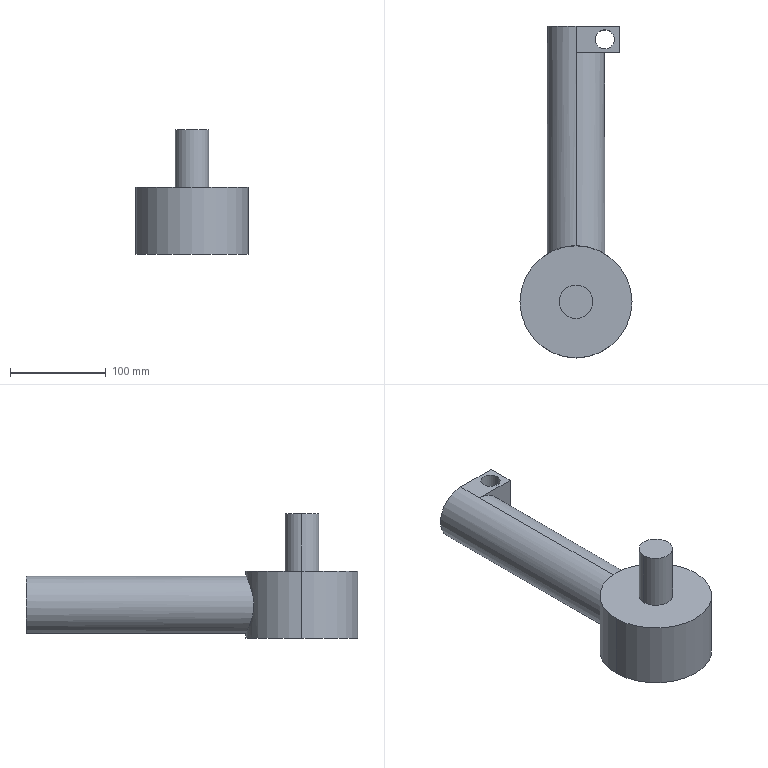Part | SolidWorks | features ICE 4, Extrusion 1 | 1 solid | 16 faces | box 117 x 346.5 x 130 mm | volume 1482010 mm3 | cylinder 8 | plane 8 | commonest cylinder face diameters 20 x2 35 x2 60 x2 117 x2
STEP:
#1=CARTESIAN_POINT('',(40.,274.,65.));
#2=VERTEX_POINT('',#1);
#3=CARTESIAN_POINT('',(20.,274.,65.));
#4=VERTEX_POINT('',#3);
#5=CARTESIAN_POINT('',(30.,274.,65.));
#6=DIRECTION('',(0.,0.,-1.));
#7=DIRECTION('',(-1.,0.,0.));
#8=AXIS2_PLACEMENT_3D('',#5,#6,#7);
#9=CIRCLE('',#8,10.);
#10=EDGE_CURVE('',#2,#4,#9,.T.);
#11=ORIENTED_EDGE('',*,*,#10,.F.);
#12=CARTESIAN_POINT('',(40.,274.,5.));
#13=VERTEX_POINT('',#12);
#14=CARTESIAN_POINT('',(40.,274.,130.));
#15=DIRECTION('',(0.,0.,-1.));
#16=VECTOR('',#15,1000.);
#17=LINE('',#14,#16);
#18=EDGE_CURVE('',#2,#13,#17,.T.);
#19=ORIENTED_EDGE('',*,*,#18,.T.);
#20=CARTESIAN_POINT('',(20.,274.,5.));
#21=VERTEX_POINT('',#20);
#22=CARTESIAN_POINT('',(30.,274.,5.));
#23=DIRECTION('',(0.,0.,-1.));
#24=DIRECTION('',(-1.,0.,0.));
#25=AXIS2_PLACEMENT_3D('',#22,#23,#24);
#26=CIRCLE('',#25,10.);
#27=EDGE_CURVE('',#13,#21,#26,.T.);
#28=ORIENTED_EDGE('',*,*,#27,.T.);
#29=CARTESIAN_POINT('',(20.,274.,130.));
#30=DIRECTION('',(0.,0.,-1.));
#31=VECTOR('',#30,1000.);
#32=LINE('',#29,#31);
#33=EDGE_CURVE('',#4,#21,#32,.T.);
#34=ORIENTED_EDGE('',*,*,#33,.F.);
#35=EDGE_LOOP('',(#11,#19,#28,#34));
#36=FACE_OUTER_BOUND('',#35,.T.);
#37=CARTESIAN_POINT('',(30.,274.,130.));
#38=DIRECTION('',(0.,0.,-1.));
#39=DIRECTION('',(-1.,0.,0.));
#40=AXIS2_PLACEMENT_3D('',#37,#38,#39);
#41=CYLINDRICAL_SURFACE('',#40,10.);
#42=ADVANCED_FACE('',(#36),#41,.F.);
#43=CARTESIAN_POINT('',(17.5,0.,130.));
#44=VERTEX_POINT('',#43);
#45=CARTESIAN_POINT('',(-17.5,0.,130.));
#46=VERTEX_POINT('',#45);
#47=CARTESIAN_POINT('',(0.,0.,130.));
#48=DIRECTION('',(0.,0.,1.));
#49=DIRECTION('',(1.,0.,0.));
#50=AXIS2_PLACEMENT_3D('',#47,#48,#49);
#51=CIRCLE('',#50,17.5);
#52=EDGE_CURVE('',#44,#46,#51,.T.);
#53=ORIENTED_EDGE('',*,*,#52,.F.);
#54=CARTESIAN_POINT('',(17.5,0.,70.));
#55=VERTEX_POINT('',#54);
#56=CARTESIAN_POINT('',(17.5,0.,130.));
#57=DIRECTION('',(0.,0.,-1.));
#58=VECTOR('',#57,1000.);
#59=LINE('',#56,#58);
#60=EDGE_CURVE('',#44,#55,#59,.T.);
#61=ORIENTED_EDGE('',*,*,#60,.T.);
#62=CARTESIAN_POINT('',(-17.5,0.,70.));
#63=VERTEX_POINT('',#62);
#64=CARTESIAN_POINT('',(0.,0.,70.));
#65=DIRECTION('',(0.,0.,1.));
#66=DIRECTION('',(1.,0.,0.));
#67=AXIS2_PLACEMENT_3D('',#64,#65,#66);
#68=CIRCLE('',#67,17.5);
#69=EDGE_CURVE('',#55,#63,#68,.T.);
#70=ORIENTED_EDGE('',*,*,#69,.T.);
#71=CARTESIAN_POINT('',(-17.5,0.,130.));
#72=DIRECTION('',(0.,0.,-1.));
#73=VECTOR('',#72,1000.);
#74=LINE('',#71,#73);
#75=EDGE_CURVE('',#46,#63,#74,.T.);
#76=ORIENTED_EDGE('',*,*,#75,.F.);
#77=EDGE_LOOP('',(#53,#61,#70,#76));
#78=FACE_OUTER_BOUND('',#77,.T.);
#79=CARTESIAN_POINT('',(0.,0.,130.));
#80=DIRECTION('',(0.,0.,-1.));
#81=DIRECTION('',(-1.,0.,0.));
#82=AXIS2_PLACEMENT_3D('',#79,#80,#81);
#83=CYLINDRICAL_SURFACE('',#82,17.5);
#84=ADVANCED_FACE('',(#78),#83,.T.);
#85=CARTESIAN_POINT('',(0.,260.,65.));
#86=VERTEX_POINT('',#85);
#87=CARTESIAN_POINT('',(0.,260.,5.));
#88=VERTEX_POINT('',#87);
#89=CARTESIAN_POINT('',(0.,260.,35.));
#90=DIRECTION('',(0.,1.,0.));
#91=DIRECTION('',(0.,0.,1.));
#92=AXIS2_PLACEMENT_3D('',#89,#90,#91);
#93=CIRCLE('',#92,30.);
#94=EDGE_CURVE('',#86,#88,#93,.T.);
#95=ORIENTED_EDGE('',*,*,#94,.F.);
#96=CARTESIAN_POINT('',(0.,58.5,65.));
#97=VERTEX_POINT('',#96);
#98=CARTESIAN_POINT('',(0.,260.,65.));
#99=DIRECTION('',(0.,-1.,0.));
#100=VECTOR('',#99,1000.);
#101=LINE('',#98,#100);
#102=EDGE_CURVE('',#86,#97,#101,.T.);
#103=ORIENTED_EDGE('',*,*,#102,.T.);
#104=CARTESIAN_POINT('',(0.,58.5,5.));
#105=VERTEX_POINT('',#104);
#106=CARTESIAN_POINT('',(0.,58.5,65.));
#107=CARTESIAN_POINT('',(0.9956,58.5,65.));
#108=CARTESIAN_POINT('',(1.997,58.475,64.95));
#109=CARTESIAN_POINT('',(4.002,58.372,64.749));
#110=CARTESIAN_POINT('',(4.989,58.295,64.599));
#111=CARTESIAN_POINT('',(7.906,57.996,64.007));
#112=CARTESIAN_POINT('',(9.794,57.704,63.425));
#113=CARTESIAN_POINT('',(13.45,56.963,61.889));
#114=CARTESIAN_POINT('',(15.161,56.526,60.959));
#115=CARTESIAN_POINT('',(17.571,55.805,59.335));
#116=CARTESIAN_POINT('',(18.348,55.554,58.755));
#117=CARTESIAN_POINT('',(19.849,55.036,57.516));
#118=CARTESIAN_POINT('',(20.565,54.771,56.863));
#119=CARTESIAN_POINT('',(22.603,53.977,54.819));
#120=CARTESIAN_POINT('',(23.822,53.443,53.337));
#121=CARTESIAN_POINT('',(25.443,52.681,50.925));
#122=CARTESIAN_POINT('',(25.95,52.432,50.084));
#123=CARTESIAN_POINT('',(26.873,51.965,48.371));
#124=CARTESIAN_POINT('',(27.291,51.746,47.495));
#125=CARTESIAN_POINT('',(28.418,51.141,44.807));
#126=CARTESIAN_POINT('',(29.,50.808,42.936));
#127=CARTESIAN_POINT('',(29.499,50.518,40.484));
#128=CARTESIAN_POINT('',(29.587,50.467,39.989));
#129=CARTESIAN_POINT('',(29.736,50.379,39.001));
#130=CARTESIAN_POINT('',(29.799,50.342,38.506));
#131=CARTESIAN_POINT('',(29.948,50.253,37.021));
#132=CARTESIAN_POINT('',(29.999,50.223,36.03));
#133=CARTESIAN_POINT('',(30.001,50.221,34.044));
#134=CARTESIAN_POINT('',(29.953,50.25,33.049));
#135=CARTESIAN_POINT('',(29.806,50.338,31.555));
#136=CARTESIAN_POINT('',(29.744,50.374,31.055));
#137=CARTESIAN_POINT('',(29.595,50.462,30.061));
#138=CARTESIAN_POINT('',(29.508,50.512,29.569));
#139=CARTESIAN_POINT('',(29.018,50.798,27.13));
#140=CARTESIAN_POINT('',(28.439,51.129,25.249));
#141=CARTESIAN_POINT('',(27.491,51.639,22.979));
#142=CARTESIAN_POINT('',(27.289,51.746,22.528));
#143=CARTESIAN_POINT('',(26.866,51.967,21.641));
#144=CARTESIAN_POINT('',(26.645,52.08,21.205));
#145=CARTESIAN_POINT('',(25.952,52.431,19.919));
#146=CARTESIAN_POINT('',(25.452,52.676,19.09));
#147=CARTESIAN_POINT('',(24.376,53.183,17.487));
#148=CARTESIAN_POINT('',(23.801,53.444,16.712));
#149=CARTESIAN_POINT('',(22.572,53.974,15.215));
#150=CARTESIAN_POINT('',(21.917,54.244,14.492));
#151=CARTESIAN_POINT('',(19.871,55.041,12.442));
#152=CARTESIAN_POINT('',(18.39,55.56,11.218));
#153=CARTESIAN_POINT('',(15.981,56.281,9.592));
#154=CARTESIAN_POINT('',(15.146,56.512,9.085));
#155=CARTESIAN_POINT('',(13.414,56.948,8.148));
#156=CARTESIAN_POINT('',(12.529,57.15,7.724));
#157=CARTESIAN_POINT('',(9.824,57.699,6.586));
#158=CARTESIAN_POINT('',(7.948,57.991,6.004));
#159=CARTESIAN_POINT('',(5.02,58.292,5.406));
#160=CARTESIAN_POINT('',(4.02,58.37,5.254));
#161=CARTESIAN_POINT('',(2.518,58.448,5.102));
#162=CARTESIAN_POINT('',(2.016,58.467,5.064));
#163=CARTESIAN_POINT('',(1.01,58.493,5.013));
#164=CARTESIAN_POINT('',(0.5043,58.5,5.));
#165=CARTESIAN_POINT('',(0.,58.5,5.));
#166=B_SPLINE_CURVE_WITH_KNOTS('',3,(#106,#107,#108,#109,#110,#111,#112,#113,#114,#115,#116,#117,#118,#119,#120,#121,#122,#123,#124,#125,#126,#127,#128,#129,#130,#131,#132,#133,#134,#135,#136,#137,#138,#139,#140,#141,#142,#143,#144,#145,#146,#147,#148,#149,#150,#151,#152,#153,#154,#155,#156,#157,#158,#159,#160,#161,#162,#163,#164,#165),.UNSPECIFIED.,.F.,.F.,(4,2,2,2,2,2,2,2,2,2,2,2,2,2,2,2,2,2,2,2,2,2,2,2,2,2,2,2,2,4),(0.09553,0.0985,0.1015,0.1074,0.1134,0.1164,0.1194,0.1253,0.1283,0.1313,0.1372,0.1387,0.1402,0.1432,0.1462,0.1477,0.1492,0.1551,0.1566,0.1581,0.1611,0.1641,0.167,0.173,0.176,0.179,0.1849,0.1879,0.1894,0.1909),.UNSPECIFIED.);
#167=EDGE_CURVE('',#97,#105,#166,.T.);
#168=ORIENTED_EDGE('',*,*,#167,.T.);
#169=CARTESIAN_POINT('',(0.,260.,5.));
#170=DIRECTION('',(0.,-1.,0.));
#171=VECTOR('',#170,1000.);
#172=LINE('',#169,#171);
#173=EDGE_CURVE('',#88,#105,#172,.T.);
#174=ORIENTED_EDGE('',*,*,#173,.F.);
#175=EDGE_LOOP('',(#95,#103,#168,#174));
#176=FACE_OUTER_BOUND('',#175,.T.);
#177=CARTESIAN_POINT('',(0.,260.,35.));
#178=DIRECTION('',(0.,-1.,0.));
#179=DIRECTION('',(0.,0.,-1.));
#180=AXIS2_PLACEMENT_3D('',#177,#178,#179);
#181=CYLINDRICAL_SURFACE('',#180,30.);
#182=ADVANCED_FACE('',(#176),#181,.T.);
#183=CARTESIAN_POINT('',(0.,58.5,5.));
#184=CARTESIAN_POINT('',(-2.021,58.5,5.));
#185=CARTESIAN_POINT('',(-4.002,58.396,5.202));
#186=CARTESIAN_POINT('',(-6.917,58.098,5.791));
#187=CARTESIAN_POINT('',(-7.879,57.975,6.036));
#188=CARTESIAN_POINT('',(-9.307,57.757,6.476));
#189=CARTESIAN_POINT('',(-9.781,57.678,6.635));
#190=CARTESIAN_POINT('',(-10.712,57.513,6.973));
#191=CARTESIAN_POINT('',(-11.171,57.425,7.153));
#192=CARTESIAN_POINT('',(-13.436,56.966,8.105));
#193=CARTESIAN_POINT('',(-15.147,56.53,9.031));
#194=CARTESIAN_POINT('',(-17.17,55.925,10.394));
#195=CARTESIAN_POINT('',(-17.569,55.801,10.678));
#196=CARTESIAN_POINT('',(-18.349,55.549,11.261));
#197=CARTESIAN_POINT('',(-18.731,55.422,11.561));
#198=CARTESIAN_POINT('',(-19.849,55.035,12.484));
#199=CARTESIAN_POINT('',(-20.56,54.773,13.132));
#200=CARTESIAN_POINT('',(-21.918,54.244,14.493));
#201=CARTESIAN_POINT('',(-22.564,53.978,15.206));
#202=CARTESIAN_POINT('',(-23.484,53.581,16.325));
#203=CARTESIAN_POINT('',(-23.782,53.449,16.707));
#204=CARTESIAN_POINT('',(-24.362,53.187,17.487));
#205=CARTESIAN_POINT('',(-24.644,53.057,17.885));
#206=CARTESIAN_POINT('',(-25.995,52.421,19.9));
#207=CARTESIAN_POINT('',(-26.912,51.949,21.6));
#208=CARTESIAN_POINT('',(-28.042,51.343,24.295));
#209=CARTESIAN_POINT('',(-28.377,51.157,25.217));
#210=CARTESIAN_POINT('',(-28.816,50.911,26.64));
#211=CARTESIAN_POINT('',(-28.951,50.834,27.121));
#212=CARTESIAN_POINT('',(-29.197,50.693,28.086));
#213=CARTESIAN_POINT('',(-29.307,50.63,28.57));
#214=CARTESIAN_POINT('',(-29.798,50.344,30.999));
#215=CARTESIAN_POINT('',(-29.998,50.223,32.97));
#216=CARTESIAN_POINT('',(-30.001,50.222,35.469));
#217=CARTESIAN_POINT('',(-29.989,50.229,35.97));
#218=CARTESIAN_POINT('',(-29.939,50.258,36.977));
#219=CARTESIAN_POINT('',(-29.901,50.281,37.481));
#220=CARTESIAN_POINT('',(-29.752,50.37,38.979));
#221=CARTESIAN_POINT('',(-29.603,50.457,39.963));
#222=CARTESIAN_POINT('',(-29.211,50.685,41.906));
#223=CARTESIAN_POINT('',(-28.968,50.825,42.864));
#224=CARTESIAN_POINT('',(-28.387,51.152,44.755));
#225=CARTESIAN_POINT('',(-28.047,51.34,45.692));
#226=CARTESIAN_POINT('',(-26.906,51.952,48.413));
#227=CARTESIAN_POINT('',(-25.983,52.427,50.121));
#228=CARTESIAN_POINT('',(-24.36,53.19,52.536));
#229=CARTESIAN_POINT('',(-23.776,53.455,53.32));
#230=CARTESIAN_POINT('',(-22.545,53.985,54.816));
#231=CARTESIAN_POINT('',(-21.897,54.252,55.529));
#232=CARTESIAN_POINT('',(-19.858,55.046,57.569));
#233=CARTESIAN_POINT('',(-18.372,55.566,58.797));
#234=CARTESIAN_POINT('',(-15.12,56.538,60.985));
#235=CARTESIAN_POINT('',(-13.405,56.973,61.909));
#236=CARTESIAN_POINT('',(-10.704,57.52,63.042));
#237=CARTESIAN_POINT('',(-9.781,57.684,63.378));
#238=CARTESIAN_POINT('',(-8.362,57.901,63.815));
#239=CARTESIAN_POINT('',(-7.883,57.968,63.95));
#240=CARTESIAN_POINT('',(-6.914,58.092,64.197));
#241=CARTESIAN_POINT('',(-6.423,58.148,64.309));
#242=CARTESIAN_POINT('',(-3.973,58.398,64.803));
#243=CARTESIAN_POINT('',(-1.995,58.5,65.));
#244=CARTESIAN_POINT('',(0.,58.5,65.));
#245=B_SPLINE_CURVE_WITH_KNOTS('',3,(#183,#184,#185,#186,#187,#188,#189,#190,#191,#192,#193,#194,#195,#196,#197,#198,#199,#200,#201,#202,#203,#204,#205,#206,#207,#208,#209,#210,#211,#212,#213,#214,#215,#216,#217,#218,#219,#220,#221,#222,#223,#224,#225,#226,#227,#228,#229,#230,#231,#232,#233,#234,#235,#236,#237,#238,#239,#240,#241,#242,#243,#244),.UNSPECIFIED.,.F.,.F.,(4,2,2,2,2,2,2,2,2,2,2,2,2,2,2,2,2,2,2,2,2,2,2,2,2,2,2,2,2,2,4),(0.,0.00597,0.008956,0.01045,0.01194,0.01791,0.0194,0.0209,0.02388,0.02687,0.02836,0.02985,0.03582,0.03881,0.0403,0.04179,0.04776,0.04926,0.05075,0.05373,0.05672,0.0597,0.06567,0.06866,0.07164,0.07761,0.08358,0.08657,0.08806,0.08956,0.09553),.UNSPECIFIED.);
#246=EDGE_CURVE('',#105,#97,#245,.T.);
#247=ORIENTED_EDGE('',*,*,#246,.F.);
#248=ORIENTED_EDGE('',*,*,#167,.F.);
#249=EDGE_LOOP('',(#247,#248));
#250=FACE_BOUND('',#249,.T.);
#251=CARTESIAN_POINT('',(58.5,0.,70.));
#252=VERTEX_POINT('',#251);
#253=CARTESIAN_POINT('',(-58.5,0.,70.));
#254=VERTEX_POINT('',#253);
#255=CARTESIAN_POINT('',(0.,0.,70.));
#256=DIRECTION('',(0.,0.,1.));
#257=DIRECTION('',(1.,0.,0.));
#258=AXIS2_PLACEMENT_3D('',#255,#256,#257);
#259=CIRCLE('',#258,58.5);
#260=EDGE_CURVE('',#252,#254,#259,.T.);
#261=ORIENTED_EDGE('',*,*,#260,.F.);
#262=CARTESIAN_POINT('',(58.5,0.,0.));
#263=VERTEX_POINT('',#262);
#264=CARTESIAN_POINT('',(58.5,0.,70.));
#265=DIRECTION('',(0.,0.,-1.));
#266=VECTOR('',#265,1000.);
#267=LINE('',#264,#266);
#268=EDGE_CURVE('',#252,#263,#267,.T.);
#269=ORIENTED_EDGE('',*,*,#268,.T.);
#270=CARTESIAN_POINT('',(-58.5,0.,0.));
#271=VERTEX_POINT('',#270);
#272=CARTESIAN_POINT('',(0.,0.,0.));
#273=DIRECTION('',(0.,0.,1.));
#274=DIRECTION('',(1.,0.,0.));
#275=AXIS2_PLACEMENT_3D('',#272,#273,#274);
#276=CIRCLE('',#275,58.5);
#277=EDGE_CURVE('',#263,#271,#276,.T.);
#278=ORIENTED_EDGE('',*,*,#277,.T.);
#279=CARTESIAN_POINT('',(-58.5,0.,70.));
#280=DIRECTION('',(0.,0.,-1.));
#281=VECTOR('',#280,1000.);
#282=LINE('',#279,#281);
#283=EDGE_CURVE('',#254,#271,#282,.T.);
#284=ORIENTED_EDGE('',*,*,#283,.F.);
#285=EDGE_LOOP('',(#261,#269,#278,#284));
#286=FACE_OUTER_BOUND('',#285,.T.);
#287=CARTESIAN_POINT('',(0.,0.,70.));
#288=DIRECTION('',(0.,0.,-1.));
#289=DIRECTION('',(-1.,0.,0.));
#290=AXIS2_PLACEMENT_3D('',#287,#288,#289);
#291=CYLINDRICAL_SURFACE('',#290,58.5);
#292=ADVANCED_FACE('',(#250,#286),#291,.T.);
#293=ORIENTED_EDGE('',*,*,#268,.F.);
#294=CARTESIAN_POINT('',(0.,0.,70.));
#295=DIRECTION('',(0.,0.,1.));
#296=DIRECTION('',(1.,0.,0.));
#297=AXIS2_PLACEMENT_3D('',#294,#295,#296);
#298=CIRCLE('',#297,58.5);
#299=EDGE_CURVE('',#254,#252,#298,.T.);
#300=ORIENTED_EDGE('',*,*,#299,.F.);
#301=ORIENTED_EDGE('',*,*,#283,.T.);
#302=CARTESIAN_POINT('',(0.,0.,0.));
#303=DIRECTION('',(0.,0.,1.));
#304=DIRECTION('',(1.,0.,0.));
#305=AXIS2_PLACEMENT_3D('',#302,#303,#304);
#306=CIRCLE('',#305,58.5);
#307=EDGE_CURVE('',#271,#263,#306,.T.);
#308=ORIENTED_EDGE('',*,*,#307,.T.);
#309=EDGE_LOOP('',(#293,#300,#301,#308));
#310=FACE_OUTER_BOUND('',#309,.T.);
#311=CARTESIAN_POINT('',(0.,0.,70.));
#312=DIRECTION('',(0.,0.,-1.));
#313=DIRECTION('',(-1.,0.,0.));
#314=AXIS2_PLACEMENT_3D('',#311,#312,#313);
#315=CYLINDRICAL_SURFACE('',#314,58.5);
#316=ADVANCED_FACE('',(#310),#315,.T.);
#317=CARTESIAN_POINT('',(0.,0.,70.));
#318=DIRECTION('',(0.,0.,1.));
#319=DIRECTION('',(1.,0.,0.));
#320=AXIS2_PLACEMENT_3D('',#317,#318,#319);
#321=CIRCLE('',#320,17.5);
#322=EDGE_CURVE('',#63,#55,#321,.T.);
#323=ORIENTED_EDGE('',*,*,#322,.F.);
#324=ORIENTED_EDGE('',*,*,#69,.F.);
#325=EDGE_LOOP('',(#323,#324));
#326=FACE_BOUND('',#325,.T.);
#327=ORIENTED_EDGE('',*,*,#299,.T.);
#328=ORIENTED_EDGE('',*,*,#260,.T.);
#329=EDGE_LOOP('',(#327,#328));
#330=FACE_OUTER_BOUND('',#329,.T.);
#331=CARTESIAN_POINT('',(0.,0.,70.));
#332=DIRECTION('',(0.,0.,1.));
#333=DIRECTION('',(1.,0.,0.));
#334=AXIS2_PLACEMENT_3D('',#331,#332,#333);
#335=PLANE('',#334);
#336=ADVANCED_FACE('',(#326,#330),#335,.T.);
#337=ORIENTED_EDGE('',*,*,#307,.F.);
#338=ORIENTED_EDGE('',*,*,#277,.F.);
#339=EDGE_LOOP('',(#337,#338));
#340=FACE_OUTER_BOUND('',#339,.T.);
#341=CARTESIAN_POINT('',(0.,0.,0.));
#342=DIRECTION('',(0.,0.,1.));
#343=DIRECTION('',(1.,0.,0.));
#344=AXIS2_PLACEMENT_3D('',#341,#342,#343);
#345=PLANE('',#344);
#346=ADVANCED_FACE('',(#340),#345,.F.);
#347=ORIENTED_EDGE('',*,*,#102,.F.);
#348=CARTESIAN_POINT('',(0.,288.,65.));
#349=VERTEX_POINT('',#348);
#350=CARTESIAN_POINT('',(0.,288.,65.));
#351=DIRECTION('',(0.,-1.,0.));
#352=VECTOR('',#351,1000.);
#353=LINE('',#350,#352);
#354=EDGE_CURVE('',#349,#86,#353,.T.);
#355=ORIENTED_EDGE('',*,*,#354,.F.);
#356=CARTESIAN_POINT('',(0.,288.,5.));
#357=VERTEX_POINT('',#356);
#358=CARTESIAN_POINT('',(0.,288.,35.));
#359=DIRECTION('',(0.,1.,0.));
#360=DIRECTION('',(0.,0.,1.));
#361=AXIS2_PLACEMENT_3D('',#358,#359,#360);
#362=CIRCLE('',#361,30.);
#363=EDGE_CURVE('',#357,#349,#362,.T.);
#364=ORIENTED_EDGE('',*,*,#363,.F.);
#365=CARTESIAN_POINT('',(0.,288.,5.));
#366=DIRECTION('',(0.,-1.,0.));
#367=VECTOR('',#366,1000.);
#368=LINE('',#365,#367);
#369=EDGE_CURVE('',#357,#88,#368,.T.);
#370=ORIENTED_EDGE('',*,*,#369,.T.);
#371=ORIENTED_EDGE('',*,*,#173,.T.);
#372=ORIENTED_EDGE('',*,*,#246,.T.);
#373=EDGE_LOOP('',(#347,#355,#364,#370,#371,#372));
#374=FACE_OUTER_BOUND('',#373,.T.);
#375=CARTESIAN_POINT('',(0.,260.,35.));
#376=DIRECTION('',(0.,-1.,0.));
#377=DIRECTION('',(0.,0.,-1.));
#378=AXIS2_PLACEMENT_3D('',#375,#376,#377);
#379=CYLINDRICAL_SURFACE('',#378,30.);
#380=ADVANCED_FACE('',(#374),#379,.T.);
#381=CARTESIAN_POINT('',(45.,260.,65.));
#382=VERTEX_POINT('',#381);
#383=CARTESIAN_POINT('',(0.,260.,65.));
#384=DIRECTION('',(1.,0.,0.));
#385=VECTOR('',#384,1000.);
#386=LINE('',#383,#385);
#387=EDGE_CURVE('',#86,#382,#386,.T.);
#388=ORIENTED_EDGE('',*,*,#387,.F.);
#389=ORIENTED_EDGE('',*,*,#94,.T.);
#390=CARTESIAN_POINT('',(45.,260.,5.));
#391=VERTEX_POINT('',#390);
#392=CARTESIAN_POINT('',(0.,260.,5.));
#393=DIRECTION('',(-1.,0.,0.));
#394=VECTOR('',#393,1000.);
#395=LINE('',#392,#394);
#396=EDGE_CURVE('',#391,#88,#395,.T.);
#397=ORIENTED_EDGE('',*,*,#396,.F.);
#398=CARTESIAN_POINT('',(45.,260.,65.));
#399=DIRECTION('',(0.,0.,-1.));
#400=VECTOR('',#399,1000.);
#401=LINE('',#398,#400);
#402=EDGE_CURVE('',#382,#391,#401,.T.);
#403=ORIENTED_EDGE('',*,*,#402,.F.);
#404=EDGE_LOOP('',(#388,#389,#397,#403));
#405=FACE_OUTER_BOUND('',#404,.T.);
#406=CARTESIAN_POINT('',(0.,260.,35.));
#407=DIRECTION('',(0.,1.,0.));
#408=DIRECTION('',(0.,0.,1.));
#409=AXIS2_PLACEMENT_3D('',#406,#407,#408);
#410=PLANE('',#409);
#411=ADVANCED_FACE('',(#405),#410,.F.);
#412=CARTESIAN_POINT('',(30.,274.,65.));
#413=DIRECTION('',(0.,0.,-1.));
#414=DIRECTION('',(-1.,0.,0.));
#415=AXIS2_PLACEMENT_3D('',#412,#413,#414);
#416=CIRCLE('',#415,10.);
#417=EDGE_CURVE('',#4,#2,#416,.T.);
#418=ORIENTED_EDGE('',*,*,#417,.T.);
#419=ORIENTED_EDGE('',*,*,#10,.T.);
#420=EDGE_LOOP('',(#418,#419));
#421=FACE_BOUND('',#420,.T.);
#422=ORIENTED_EDGE('',*,*,#387,.T.);
#423=CARTESIAN_POINT('',(45.,288.,65.));
#424=VERTEX_POINT('',#423);
#425=CARTESIAN_POINT('',(45.,288.,65.));
#426=DIRECTION('',(0.,-1.,0.));
#427=VECTOR('',#426,1000.);
#428=LINE('',#425,#427);
#429=EDGE_CURVE('',#424,#382,#428,.T.);
#430=ORIENTED_EDGE('',*,*,#429,.F.);
#431=CARTESIAN_POINT('',(0.,288.,65.));
#432=DIRECTION('',(1.,0.,0.));
#433=VECTOR('',#432,1000.);
#434=LINE('',#431,#433);
#435=EDGE_CURVE('',#349,#424,#434,.T.);
#436=ORIENTED_EDGE('',*,*,#435,.F.);
#437=ORIENTED_EDGE('',*,*,#354,.T.);
#438=EDGE_LOOP('',(#422,#430,#436,#437));
#439=FACE_OUTER_BOUND('',#438,.T.);
#440=CARTESIAN_POINT('',(0.,288.,65.));
#441=DIRECTION('',(0.,0.,-1.));
#442=DIRECTION('',(-1.,0.,0.));
#443=AXIS2_PLACEMENT_3D('',#440,#441,#442);
#444=PLANE('',#443);
#445=ADVANCED_FACE('',(#421,#439),#444,.F.);
#446=ORIENTED_EDGE('',*,*,#402,.T.);
#447=CARTESIAN_POINT('',(45.,288.,5.));
#448=VERTEX_POINT('',#447);
#449=CARTESIAN_POINT('',(45.,288.,5.));
#450=DIRECTION('',(0.,-1.,0.));
#451=VECTOR('',#450,1000.);
#452=LINE('',#449,#451);
#453=EDGE_CURVE('',#448,#391,#452,.T.);
#454=ORIENTED_EDGE('',*,*,#453,.F.);
#455=CARTESIAN_POINT('',(45.,288.,65.));
#456=DIRECTION('',(0.,0.,-1.));
#457=VECTOR('',#456,1000.);
#458=LINE('',#455,#457);
#459=EDGE_CURVE('',#424,#448,#458,.T.);
#460=ORIENTED_EDGE('',*,*,#459,.F.);
#461=ORIENTED_EDGE('',*,*,#429,.T.);
#462=EDGE_LOOP('',(#446,#454,#460,#461));
#463=FACE_OUTER_BOUND('',#462,.T.);
#464=CARTESIAN_POINT('',(45.,288.,65.));
#465=DIRECTION('',(-1.,0.,0.));
#466=DIRECTION('',(0.,0.,1.));
#467=AXIS2_PLACEMENT_3D('',#464,#465,#466);
#468=PLANE('',#467);
#469=ADVANCED_FACE('',(#463),#468,.F.);
#470=CARTESIAN_POINT('',(30.,274.,5.));
#471=DIRECTION('',(0.,0.,-1.));
#472=DIRECTION('',(-1.,0.,0.));
#473=AXIS2_PLACEMENT_3D('',#470,#471,#472);
#474=CIRCLE('',#473,10.);
#475=EDGE_CURVE('',#21,#13,#474,.T.);
#476=ORIENTED_EDGE('',*,*,#475,.F.);
#477=ORIENTED_EDGE('',*,*,#27,.F.);
#478=EDGE_LOOP('',(#476,#477));
#479=FACE_BOUND('',#478,.T.);
#480=ORIENTED_EDGE('',*,*,#396,.T.);
#481=ORIENTED_EDGE('',*,*,#369,.F.);
#482=CARTESIAN_POINT('',(0.,288.,5.));
#483=DIRECTION('',(-1.,0.,0.));
#484=VECTOR('',#483,1000.);
#485=LINE('',#482,#484);
#486=EDGE_CURVE('',#448,#357,#485,.T.);
#487=ORIENTED_EDGE('',*,*,#486,.F.);
#488=ORIENTED_EDGE('',*,*,#453,.T.);
#489=EDGE_LOOP('',(#480,#481,#487,#488));
#490=FACE_OUTER_BOUND('',#489,.T.);
#491=CARTESIAN_POINT('',(0.,288.,5.));
#492=DIRECTION('',(0.,0.,1.));
#493=DIRECTION('',(1.,0.,0.));
#494=AXIS2_PLACEMENT_3D('',#491,#492,#493);
#495=PLANE('',#494);
#496=ADVANCED_FACE('',(#479,#490),#495,.F.);
#497=ORIENTED_EDGE('',*,*,#363,.T.);
#498=ORIENTED_EDGE('',*,*,#435,.T.);
#499=ORIENTED_EDGE('',*,*,#459,.T.);
#500=ORIENTED_EDGE('',*,*,#486,.T.);
#501=EDGE_LOOP('',(#497,#498,#499,#500));
#502=FACE_OUTER_BOUND('',#501,.T.);
#503=CARTESIAN_POINT('',(0.,288.,35.));
#504=DIRECTION('',(0.,1.,0.));
#505=DIRECTION('',(0.,0.,1.));
#506=AXIS2_PLACEMENT_3D('',#503,#504,#505);
#507=PLANE('',#506);
#508=ADVANCED_FACE('',(#502),#507,.T.);
#509=ORIENTED_EDGE('',*,*,#60,.F.);
#510=CARTESIAN_POINT('',(0.,0.,130.));
#511=DIRECTION('',(0.,0.,1.));
#512=DIRECTION('',(1.,0.,0.));
#513=AXIS2_PLACEMENT_3D('',#510,#511,#512);
#514=CIRCLE('',#513,17.5);
#515=EDGE_CURVE('',#46,#44,#514,.T.);
#516=ORIENTED_EDGE('',*,*,#515,.F.);
#517=ORIENTED_EDGE('',*,*,#75,.T.);
#518=ORIENTED_EDGE('',*,*,#322,.T.);
#519=EDGE_LOOP('',(#509,#516,#517,#518));
#520=FACE_OUTER_BOUND('',#519,.T.);
#521=CARTESIAN_POINT('',(0.,0.,130.));
#522=DIRECTION('',(0.,0.,-1.));
#523=DIRECTION('',(-1.,0.,0.));
#524=AXIS2_PLACEMENT_3D('',#521,#522,#523);
#525=CYLINDRICAL_SURFACE('',#524,17.5);
#526=ADVANCED_FACE('',(#520),#525,.T.);
#527=ORIENTED_EDGE('',*,*,#515,.T.);
#528=ORIENTED_EDGE('',*,*,#52,.T.);
#529=EDGE_LOOP('',(#527,#528));
#530=FACE_OUTER_BOUND('',#529,.T.);
#531=CARTESIAN_POINT('',(0.,0.,130.));
#532=DIRECTION('',(0.,0.,1.));
#533=DIRECTION('',(1.,0.,0.));
#534=AXIS2_PLACEMENT_3D('',#531,#532,#533);
#535=PLANE('',#534);
#536=ADVANCED_FACE('',(#530),#535,.T.);
#537=ORIENTED_EDGE('',*,*,#18,.F.);
#538=ORIENTED_EDGE('',*,*,#417,.F.);
#539=ORIENTED_EDGE('',*,*,#33,.T.);
#540=ORIENTED_EDGE('',*,*,#475,.T.);
#541=EDGE_LOOP('',(#537,#538,#539,#540));
#542=FACE_OUTER_BOUND('',#541,.T.);
#543=CARTESIAN_POINT('',(30.,274.,130.));
#544=DIRECTION('',(0.,0.,-1.));
#545=DIRECTION('',(-1.,0.,0.));
#546=AXIS2_PLACEMENT_3D('',#543,#544,#545);
#547=CYLINDRICAL_SURFACE('',#546,10.);
#548=ADVANCED_FACE('',(#542),#547,.F.);
#549=CLOSED_SHELL('',(#42,#84,#182,#292,#316,#336,#346,#380,#411,#445,#469,#496,#508,#526,#536,#548));
#550=MANIFOLD_SOLID_BREP('',#549);
#551=CARTESIAN_POINT('',(0.,0.,0.));
#552=DIRECTION('',(0.,0.,1.));
#553=DIRECTION('',(1.,0.,0.));
#554=AXIS2_PLACEMENT_3D('',#551,#552,#553);
#555=(LENGTH_UNIT()NAMED_UNIT(*)SI_UNIT(.MILLI.,.METRE.));
#556=UNCERTAINTY_MEASURE_WITH_UNIT(LENGTH_MEASURE(0.00001),#555,'','');
#557=(NAMED_UNIT(*)PLANE_ANGLE_UNIT()SI_UNIT($,.RADIAN.));
#558=(NAMED_UNIT(*)SI_UNIT($,.STERADIAN.)SOLID_ANGLE_UNIT());
#559=(GEOMETRIC_REPRESENTATION_CONTEXT(3)GLOBAL_UNCERTAINTY_ASSIGNED_CONTEXT((#556))GLOBAL_UNIT_ASSIGNED_CONTEXT((#555,#557,#558))REPRESENTATION_CONTEXT('',''));
#560=ADVANCED_BREP_SHAPE_REPRESENTATION('',(#550,#554),#559);